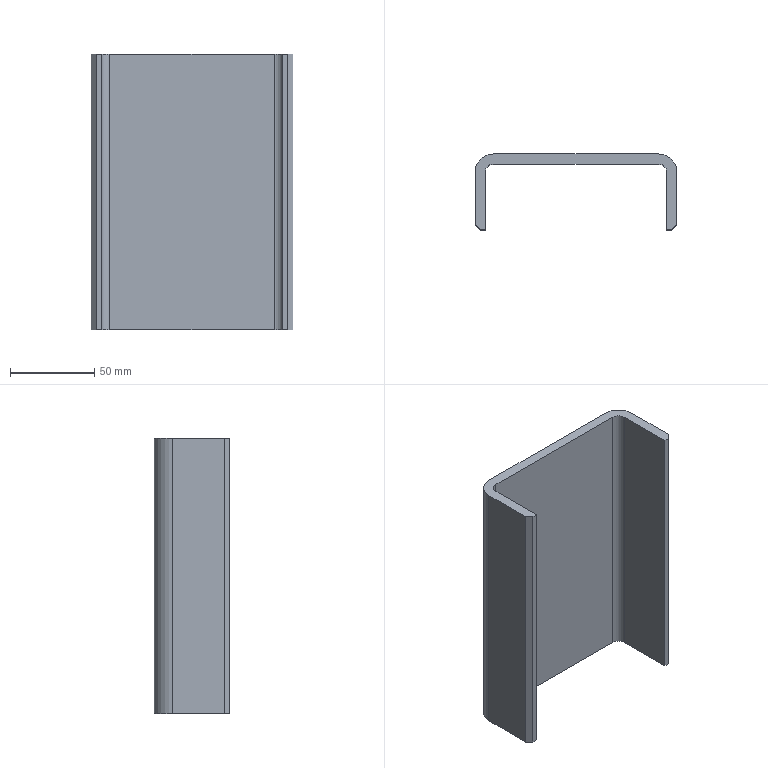Part | STEP file | VD-SYL0380DJ1006_1_1_2-2_VD-SYL | 1 solid | 16 faces | box 120 x 45 x 164 mm | volume 186599 mm3 | plane 12 | cylinder 4 | commonest cylinder face diameters 10 x2 22 x2
STEP:
#1=CARTESIAN_POINT('',(-49.,22.5,82.));
#2=VERTEX_POINT('',#1);
#3=CARTESIAN_POINT('',(-49.,22.5,-82.));
#4=VERTEX_POINT('',#3);
#5=CARTESIAN_POINT('',(-49.,22.5,82.));
#6=DIRECTION('',(0.,0.,-1.));
#7=VECTOR('',#6,1000.);
#8=LINE('',#5,#7);
#9=EDGE_CURVE('',#2,#4,#8,.T.);
#10=ORIENTED_EDGE('',*,*,#9,.T.);
#11=CARTESIAN_POINT('',(-60.,11.5,-82.));
#12=VERTEX_POINT('',#11);
#13=CARTESIAN_POINT('',(-49.,11.5,-82.));
#14=DIRECTION('',(0.,0.,-1.));
#15=DIRECTION('',(-1.,0.,0.));
#16=AXIS2_PLACEMENT_3D('',#13,#14,#15);
#17=CIRCLE('',#16,11.);
#18=EDGE_CURVE('',#12,#4,#17,.T.);
#19=ORIENTED_EDGE('',*,*,#18,.F.);
#20=CARTESIAN_POINT('',(-60.,11.5,82.));
#21=VERTEX_POINT('',#20);
#22=CARTESIAN_POINT('',(-60.,11.5,-82.));
#23=DIRECTION('',(0.,0.,1.));
#24=VECTOR('',#23,1000.);
#25=LINE('',#22,#24);
#26=EDGE_CURVE('',#12,#21,#25,.T.);
#27=ORIENTED_EDGE('',*,*,#26,.T.);
#28=CARTESIAN_POINT('',(-49.,11.5,82.));
#29=DIRECTION('',(0.,0.,1.));
#30=DIRECTION('',(0.,1.,0.));
#31=AXIS2_PLACEMENT_3D('',#28,#29,#30);
#32=CIRCLE('',#31,11.);
#33=EDGE_CURVE('',#2,#21,#32,.T.);
#34=ORIENTED_EDGE('',*,*,#33,.F.);
#35=EDGE_LOOP('',(#10,#19,#27,#34));
#36=FACE_OUTER_BOUND('',#35,.T.);
#37=CARTESIAN_POINT('',(-49.,11.5,295.79));
#38=DIRECTION('',(0.,0.,-1.));
#39=DIRECTION('',(-1.,0.,0.));
#40=AXIS2_PLACEMENT_3D('',#37,#38,#39);
#41=CYLINDRICAL_SURFACE('',#40,11.);
#42=ADVANCED_FACE('',(#36),#41,.T.);
#43=CARTESIAN_POINT('',(-60.,-19.5,82.));
#44=VERTEX_POINT('',#43);
#45=CARTESIAN_POINT('',(-60.,-19.5,-82.));
#46=VERTEX_POINT('',#45);
#47=CARTESIAN_POINT('',(-60.,-19.5,82.));
#48=DIRECTION('',(0.,0.,-1.));
#49=VECTOR('',#48,1000.);
#50=LINE('',#47,#49);
#51=EDGE_CURVE('',#44,#46,#50,.T.);
#52=ORIENTED_EDGE('',*,*,#51,.F.);
#53=CARTESIAN_POINT('',(-60.,11.5,82.));
#54=DIRECTION('',(0.,-1.,0.));
#55=VECTOR('',#54,1000.);
#56=LINE('',#53,#55);
#57=EDGE_CURVE('',#21,#44,#56,.T.);
#58=ORIENTED_EDGE('',*,*,#57,.F.);
#59=ORIENTED_EDGE('',*,*,#26,.F.);
#60=CARTESIAN_POINT('',(-60.,-19.5,-82.));
#61=DIRECTION('',(0.,1.,0.));
#62=VECTOR('',#61,1000.);
#63=LINE('',#60,#62);
#64=EDGE_CURVE('',#46,#12,#63,.T.);
#65=ORIENTED_EDGE('',*,*,#64,.F.);
#66=EDGE_LOOP('',(#52,#58,#59,#65));
#67=FACE_OUTER_BOUND('',#66,.T.);
#68=CARTESIAN_POINT('',(-60.,22.5,-82.));
#69=DIRECTION('',(-1.,0.,0.));
#70=DIRECTION('',(0.,0.,1.));
#71=AXIS2_PLACEMENT_3D('',#68,#69,#70);
#72=PLANE('',#71);
#73=ADVANCED_FACE('',(#67),#72,.T.);
#74=CARTESIAN_POINT('',(-57.,-22.5,-82.));
#75=VERTEX_POINT('',#74);
#76=CARTESIAN_POINT('',(-57.,-22.5,-82.));
#77=DIRECTION('',(-0.7071,0.7071,0.));
#78=VECTOR('',#77,1000.);
#79=LINE('',#76,#78);
#80=EDGE_CURVE('',#75,#46,#79,.T.);
#81=ORIENTED_EDGE('',*,*,#80,.F.);
#82=CARTESIAN_POINT('',(-57.,-22.5,82.));
#83=VERTEX_POINT('',#82);
#84=CARTESIAN_POINT('',(-57.,-22.5,82.));
#85=DIRECTION('',(0.,0.,-1.));
#86=VECTOR('',#85,1000.);
#87=LINE('',#84,#86);
#88=EDGE_CURVE('',#83,#75,#87,.T.);
#89=ORIENTED_EDGE('',*,*,#88,.F.);
#90=CARTESIAN_POINT('',(-60.,-19.5,82.));
#91=DIRECTION('',(0.7071,-0.7071,0.));
#92=VECTOR('',#91,1000.);
#93=LINE('',#90,#92);
#94=EDGE_CURVE('',#44,#83,#93,.T.);
#95=ORIENTED_EDGE('',*,*,#94,.F.);
#96=ORIENTED_EDGE('',*,*,#51,.T.);
#97=EDGE_LOOP('',(#81,#89,#95,#96));
#98=FACE_OUTER_BOUND('',#97,.T.);
#99=CARTESIAN_POINT('',(-58.5,-21.,0.));
#100=DIRECTION('',(-0.7071,-0.7071,0.));
#101=DIRECTION('',(-0.7071,0.7071,0.));
#102=AXIS2_PLACEMENT_3D('',#99,#100,#101);
#103=PLANE('',#102);
#104=ADVANCED_FACE('',(#98),#103,.T.);
#105=ORIENTED_EDGE('',*,*,#88,.T.);
#106=CARTESIAN_POINT('',(-54.,-22.5,-82.));
#107=VERTEX_POINT('',#106);
#108=CARTESIAN_POINT('',(-57.,-22.5,-82.));
#109=DIRECTION('',(1.,0.,0.));
#110=VECTOR('',#109,1000.);
#111=LINE('',#108,#110);
#112=EDGE_CURVE('',#75,#107,#111,.T.);
#113=ORIENTED_EDGE('',*,*,#112,.T.);
#114=CARTESIAN_POINT('',(-54.,-22.5,82.));
#115=VERTEX_POINT('',#114);
#116=CARTESIAN_POINT('',(-54.,-22.5,82.));
#117=DIRECTION('',(0.,0.,-1.));
#118=VECTOR('',#117,1000.);
#119=LINE('',#116,#118);
#120=EDGE_CURVE('',#115,#107,#119,.T.);
#121=ORIENTED_EDGE('',*,*,#120,.F.);
#122=CARTESIAN_POINT('',(-57.,-22.5,82.));
#123=DIRECTION('',(1.,0.,0.));
#124=VECTOR('',#123,1000.);
#125=LINE('',#122,#124);
#126=EDGE_CURVE('',#83,#115,#125,.T.);
#127=ORIENTED_EDGE('',*,*,#126,.F.);
#128=EDGE_LOOP('',(#105,#113,#121,#127));
#129=FACE_OUTER_BOUND('',#128,.T.);
#130=CARTESIAN_POINT('',(-57.,-22.5,0.));
#131=DIRECTION('',(0.,-1.,0.));
#132=DIRECTION('',(0.,0.,-1.));
#133=AXIS2_PLACEMENT_3D('',#130,#131,#132);
#134=PLANE('',#133);
#135=ADVANCED_FACE('',(#129),#134,.T.);
#136=CARTESIAN_POINT('',(-54.,11.5,-82.));
#137=VERTEX_POINT('',#136);
#138=CARTESIAN_POINT('',(-54.,-22.5,-82.));
#139=DIRECTION('',(0.,1.,0.));
#140=VECTOR('',#139,1000.);
#141=LINE('',#138,#140);
#142=EDGE_CURVE('',#107,#137,#141,.T.);
#143=ORIENTED_EDGE('',*,*,#142,.T.);
#144=CARTESIAN_POINT('',(-54.,11.5,82.));
#145=VERTEX_POINT('',#144);
#146=CARTESIAN_POINT('',(-54.,11.5,82.));
#147=DIRECTION('',(0.,0.,-1.));
#148=VECTOR('',#147,1000.);
#149=LINE('',#146,#148);
#150=EDGE_CURVE('',#145,#137,#149,.T.);
#151=ORIENTED_EDGE('',*,*,#150,.F.);
#152=CARTESIAN_POINT('',(-54.,-22.5,82.));
#153=DIRECTION('',(0.,1.,0.));
#154=VECTOR('',#153,1000.);
#155=LINE('',#152,#154);
#156=EDGE_CURVE('',#115,#145,#155,.T.);
#157=ORIENTED_EDGE('',*,*,#156,.F.);
#158=ORIENTED_EDGE('',*,*,#120,.T.);
#159=EDGE_LOOP('',(#143,#151,#157,#158));
#160=FACE_OUTER_BOUND('',#159,.T.);
#161=CARTESIAN_POINT('',(-54.,22.5,-82.));
#162=DIRECTION('',(-1.,0.,0.));
#163=DIRECTION('',(0.,0.,1.));
#164=AXIS2_PLACEMENT_3D('',#161,#162,#163);
#165=PLANE('',#164);
#166=ADVANCED_FACE('',(#160),#165,.F.);
#167=CARTESIAN_POINT('',(-49.,16.5,-82.));
#168=VERTEX_POINT('',#167);
#169=CARTESIAN_POINT('',(-49.,11.5,-82.));
#170=DIRECTION('',(0.,0.,1.));
#171=DIRECTION('',(0.,1.,0.));
#172=AXIS2_PLACEMENT_3D('',#169,#170,#171);
#173=CIRCLE('',#172,5.);
#174=EDGE_CURVE('',#168,#137,#173,.T.);
#175=ORIENTED_EDGE('',*,*,#174,.F.);
#176=CARTESIAN_POINT('',(-49.,16.5,82.));
#177=VERTEX_POINT('',#176);
#178=CARTESIAN_POINT('',(-49.,16.5,-82.));
#179=DIRECTION('',(0.,0.,1.));
#180=VECTOR('',#179,1000.);
#181=LINE('',#178,#180);
#182=EDGE_CURVE('',#168,#177,#181,.T.);
#183=ORIENTED_EDGE('',*,*,#182,.T.);
#184=CARTESIAN_POINT('',(-49.,11.5,82.));
#185=DIRECTION('',(0.,0.,-1.));
#186=DIRECTION('',(-1.,0.,0.));
#187=AXIS2_PLACEMENT_3D('',#184,#185,#186);
#188=CIRCLE('',#187,5.);
#189=EDGE_CURVE('',#145,#177,#188,.T.);
#190=ORIENTED_EDGE('',*,*,#189,.F.);
#191=ORIENTED_EDGE('',*,*,#150,.T.);
#192=EDGE_LOOP('',(#175,#183,#190,#191));
#193=FACE_OUTER_BOUND('',#192,.T.);
#194=CARTESIAN_POINT('',(-49.,11.5,295.79));
#195=DIRECTION('',(0.,0.,-1.));
#196=DIRECTION('',(-1.,0.,0.));
#197=AXIS2_PLACEMENT_3D('',#194,#195,#196);
#198=CYLINDRICAL_SURFACE('',#197,5.);
#199=ADVANCED_FACE('',(#193),#198,.F.);
#200=CARTESIAN_POINT('',(54.,11.5,82.));
#201=VERTEX_POINT('',#200);
#202=CARTESIAN_POINT('',(54.,-22.5,82.));
#203=VERTEX_POINT('',#202);
#204=CARTESIAN_POINT('',(54.,11.5,82.));
#205=DIRECTION('',(0.,-1.,0.));
#206=VECTOR('',#205,1000.);
#207=LINE('',#204,#206);
#208=EDGE_CURVE('',#201,#203,#207,.T.);
#209=ORIENTED_EDGE('',*,*,#208,.F.);
#210=CARTESIAN_POINT('',(54.,11.5,-82.));
#211=VERTEX_POINT('',#210);
#212=CARTESIAN_POINT('',(54.,11.5,-82.));
#213=DIRECTION('',(0.,0.,1.));
#214=VECTOR('',#213,1000.);
#215=LINE('',#212,#214);
#216=EDGE_CURVE('',#211,#201,#215,.T.);
#217=ORIENTED_EDGE('',*,*,#216,.F.);
#218=CARTESIAN_POINT('',(54.,-22.5,-82.));
#219=VERTEX_POINT('',#218);
#220=CARTESIAN_POINT('',(54.,11.5,-82.));
#221=DIRECTION('',(0.,-1.,0.));
#222=VECTOR('',#221,1000.);
#223=LINE('',#220,#222);
#224=EDGE_CURVE('',#211,#219,#223,.T.);
#225=ORIENTED_EDGE('',*,*,#224,.T.);
#226=CARTESIAN_POINT('',(54.,-22.5,-82.));
#227=DIRECTION('',(0.,0.,1.));
#228=VECTOR('',#227,1000.);
#229=LINE('',#226,#228);
#230=EDGE_CURVE('',#219,#203,#229,.T.);
#231=ORIENTED_EDGE('',*,*,#230,.T.);
#232=EDGE_LOOP('',(#209,#217,#225,#231));
#233=FACE_OUTER_BOUND('',#232,.T.);
#234=CARTESIAN_POINT('',(54.,-22.5,-82.));
#235=DIRECTION('',(1.,0.,0.));
#236=DIRECTION('',(0.,1.,0.));
#237=AXIS2_PLACEMENT_3D('',#234,#235,#236);
#238=PLANE('',#237);
#239=ADVANCED_FACE('',(#233),#238,.F.);
#240=CARTESIAN_POINT('',(57.,-22.5,-82.));
#241=VERTEX_POINT('',#240);
#242=CARTESIAN_POINT('',(54.,-22.5,-82.));
#243=DIRECTION('',(1.,0.,0.));
#244=VECTOR('',#243,1000.);
#245=LINE('',#242,#244);
#246=EDGE_CURVE('',#219,#241,#245,.T.);
#247=ORIENTED_EDGE('',*,*,#246,.T.);
#248=CARTESIAN_POINT('',(57.,-22.5,82.));
#249=VERTEX_POINT('',#248);
#250=CARTESIAN_POINT('',(57.,-22.5,-82.));
#251=DIRECTION('',(0.,0.,1.));
#252=VECTOR('',#251,1000.);
#253=LINE('',#250,#252);
#254=EDGE_CURVE('',#241,#249,#253,.T.);
#255=ORIENTED_EDGE('',*,*,#254,.T.);
#256=CARTESIAN_POINT('',(54.,-22.5,82.));
#257=DIRECTION('',(1.,0.,0.));
#258=VECTOR('',#257,1000.);
#259=LINE('',#256,#258);
#260=EDGE_CURVE('',#203,#249,#259,.T.);
#261=ORIENTED_EDGE('',*,*,#260,.F.);
#262=ORIENTED_EDGE('',*,*,#230,.F.);
#263=EDGE_LOOP('',(#247,#255,#261,#262));
#264=FACE_OUTER_BOUND('',#263,.T.);
#265=CARTESIAN_POINT('',(57.,-22.5,0.));
#266=DIRECTION('',(0.,1.,0.));
#267=DIRECTION('',(1.,0.,0.));
#268=AXIS2_PLACEMENT_3D('',#265,#266,#267);
#269=PLANE('',#268);
#270=ADVANCED_FACE('',(#264),#269,.F.);
#271=CARTESIAN_POINT('',(60.,-19.5,-82.));
#272=VERTEX_POINT('',#271);
#273=CARTESIAN_POINT('',(60.,-19.5,-82.));
#274=DIRECTION('',(-0.7071,-0.7071,0.));
#275=VECTOR('',#274,1000.);
#276=LINE('',#273,#275);
#277=EDGE_CURVE('',#272,#241,#276,.T.);
#278=ORIENTED_EDGE('',*,*,#277,.F.);
#279=CARTESIAN_POINT('',(60.,-19.5,82.));
#280=VERTEX_POINT('',#279);
#281=CARTESIAN_POINT('',(60.,-19.5,-82.));
#282=DIRECTION('',(0.,0.,1.));
#283=VECTOR('',#282,1000.);
#284=LINE('',#281,#283);
#285=EDGE_CURVE('',#272,#280,#284,.T.);
#286=ORIENTED_EDGE('',*,*,#285,.T.);
#287=CARTESIAN_POINT('',(57.,-22.5,82.));
#288=DIRECTION('',(0.7071,0.7071,0.));
#289=VECTOR('',#288,1000.);
#290=LINE('',#287,#289);
#291=EDGE_CURVE('',#249,#280,#290,.T.);
#292=ORIENTED_EDGE('',*,*,#291,.F.);
#293=ORIENTED_EDGE('',*,*,#254,.F.);
#294=EDGE_LOOP('',(#278,#286,#292,#293));
#295=FACE_OUTER_BOUND('',#294,.T.);
#296=CARTESIAN_POINT('',(58.5,-21.,0.));
#297=DIRECTION('',(0.7071,-0.7071,0.));
#298=DIRECTION('',(0.,0.,-1.));
#299=AXIS2_PLACEMENT_3D('',#296,#297,#298);
#300=PLANE('',#299);
#301=ADVANCED_FACE('',(#295),#300,.T.);
#302=ORIENTED_EDGE('',*,*,#285,.F.);
#303=CARTESIAN_POINT('',(60.,11.5,-82.));
#304=VERTEX_POINT('',#303);
#305=CARTESIAN_POINT('',(60.,11.5,-82.));
#306=DIRECTION('',(0.,-1.,0.));
#307=VECTOR('',#306,1000.);
#308=LINE('',#305,#307);
#309=EDGE_CURVE('',#304,#272,#308,.T.);
#310=ORIENTED_EDGE('',*,*,#309,.F.);
#311=CARTESIAN_POINT('',(60.,11.5,82.));
#312=VERTEX_POINT('',#311);
#313=CARTESIAN_POINT('',(60.,11.5,82.));
#314=DIRECTION('',(0.,0.,-1.));
#315=VECTOR('',#314,1000.);
#316=LINE('',#313,#315);
#317=EDGE_CURVE('',#312,#304,#316,.T.);
#318=ORIENTED_EDGE('',*,*,#317,.F.);
#319=CARTESIAN_POINT('',(60.,-19.5,82.));
#320=DIRECTION('',(0.,1.,0.));
#321=VECTOR('',#320,1000.);
#322=LINE('',#319,#321);
#323=EDGE_CURVE('',#280,#312,#322,.T.);
#324=ORIENTED_EDGE('',*,*,#323,.F.);
#325=EDGE_LOOP('',(#302,#310,#318,#324));
#326=FACE_OUTER_BOUND('',#325,.T.);
#327=CARTESIAN_POINT('',(60.,-22.5,-82.));
#328=DIRECTION('',(1.,0.,0.));
#329=DIRECTION('',(0.,1.,0.));
#330=AXIS2_PLACEMENT_3D('',#327,#328,#329);
#331=PLANE('',#330);
#332=ADVANCED_FACE('',(#326),#331,.T.);
#333=ORIENTED_EDGE('',*,*,#317,.T.);
#334=CARTESIAN_POINT('',(49.,22.5,-82.));
#335=VERTEX_POINT('',#334);
#336=CARTESIAN_POINT('',(49.,11.5,-82.));
#337=DIRECTION('',(0.,0.,-1.));
#338=DIRECTION('',(0.,1.,0.));
#339=AXIS2_PLACEMENT_3D('',#336,#337,#338);
#340=CIRCLE('',#339,11.);
#341=EDGE_CURVE('',#335,#304,#340,.T.);
#342=ORIENTED_EDGE('',*,*,#341,.F.);
#343=CARTESIAN_POINT('',(49.,22.5,82.));
#344=VERTEX_POINT('',#343);
#345=CARTESIAN_POINT('',(49.,22.5,-82.));
#346=DIRECTION('',(0.,0.,1.));
#347=VECTOR('',#346,1000.);
#348=LINE('',#345,#347);
#349=EDGE_CURVE('',#335,#344,#348,.T.);
#350=ORIENTED_EDGE('',*,*,#349,.T.);
#351=CARTESIAN_POINT('',(49.,11.5,82.));
#352=DIRECTION('',(0.,0.,1.));
#353=DIRECTION('',(1.,0.,0.));
#354=AXIS2_PLACEMENT_3D('',#351,#352,#353);
#355=CIRCLE('',#354,11.);
#356=EDGE_CURVE('',#312,#344,#355,.T.);
#357=ORIENTED_EDGE('',*,*,#356,.F.);
#358=EDGE_LOOP('',(#333,#342,#350,#357));
#359=FACE_OUTER_BOUND('',#358,.T.);
#360=CARTESIAN_POINT('',(49.,11.5,295.79));
#361=DIRECTION('',(0.,0.,-1.));
#362=DIRECTION('',(-1.,0.,0.));
#363=AXIS2_PLACEMENT_3D('',#360,#361,#362);
#364=CYLINDRICAL_SURFACE('',#363,11.);
#365=ADVANCED_FACE('',(#359),#364,.T.);
#366=ORIENTED_EDGE('',*,*,#33,.T.);
#367=ORIENTED_EDGE('',*,*,#57,.T.);
#368=ORIENTED_EDGE('',*,*,#94,.T.);
#369=ORIENTED_EDGE('',*,*,#126,.T.);
#370=ORIENTED_EDGE('',*,*,#156,.T.);
#371=ORIENTED_EDGE('',*,*,#189,.T.);
#372=CARTESIAN_POINT('',(49.,16.5,82.));
#373=VERTEX_POINT('',#372);
#374=CARTESIAN_POINT('',(-49.,16.5,82.));
#375=DIRECTION('',(1.,0.,0.));
#376=VECTOR('',#375,1000.);
#377=LINE('',#374,#376);
#378=EDGE_CURVE('',#177,#373,#377,.T.);
#379=ORIENTED_EDGE('',*,*,#378,.T.);
#380=CARTESIAN_POINT('',(49.,11.5,82.));
#381=DIRECTION('',(0.,0.,-1.));
#382=DIRECTION('',(0.,1.,0.));
#383=AXIS2_PLACEMENT_3D('',#380,#381,#382);
#384=CIRCLE('',#383,5.);
#385=EDGE_CURVE('',#373,#201,#384,.T.);
#386=ORIENTED_EDGE('',*,*,#385,.T.);
#387=ORIENTED_EDGE('',*,*,#208,.T.);
#388=ORIENTED_EDGE('',*,*,#260,.T.);
#389=ORIENTED_EDGE('',*,*,#291,.T.);
#390=ORIENTED_EDGE('',*,*,#323,.T.);
#391=ORIENTED_EDGE('',*,*,#356,.T.);
#392=CARTESIAN_POINT('',(49.,22.5,82.));
#393=DIRECTION('',(-1.,0.,0.));
#394=VECTOR('',#393,1000.);
#395=LINE('',#392,#394);
#396=EDGE_CURVE('',#344,#2,#395,.T.);
#397=ORIENTED_EDGE('',*,*,#396,.T.);
#398=EDGE_LOOP('',(#366,#367,#368,#369,#370,#371,#379,#386,#387,#388,#389,#390,#391,#397));
#399=FACE_OUTER_BOUND('',#398,.T.);
#400=CARTESIAN_POINT('',(0.,19.5,82.));
#401=DIRECTION('',(0.,0.,-1.));
#402=DIRECTION('',(0.,-1.,0.));
#403=AXIS2_PLACEMENT_3D('',#400,#401,#402);
#404=PLANE('',#403);
#405=ADVANCED_FACE('',(#399),#404,.F.);
#406=CARTESIAN_POINT('',(49.,16.5,-82.));
#407=VERTEX_POINT('',#406);
#408=CARTESIAN_POINT('',(49.,11.5,-82.));
#409=DIRECTION('',(0.,0.,1.));
#410=DIRECTION('',(1.,0.,0.));
#411=AXIS2_PLACEMENT_3D('',#408,#409,#410);
#412=CIRCLE('',#411,5.);
#413=EDGE_CURVE('',#211,#407,#412,.T.);
#414=ORIENTED_EDGE('',*,*,#413,.F.);
#415=ORIENTED_EDGE('',*,*,#216,.T.);
#416=ORIENTED_EDGE('',*,*,#385,.F.);
#417=CARTESIAN_POINT('',(49.,16.5,82.));
#418=DIRECTION('',(0.,0.,-1.));
#419=VECTOR('',#418,1000.);
#420=LINE('',#417,#419);
#421=EDGE_CURVE('',#373,#407,#420,.T.);
#422=ORIENTED_EDGE('',*,*,#421,.T.);
#423=EDGE_LOOP('',(#414,#415,#416,#422));
#424=FACE_OUTER_BOUND('',#423,.T.);
#425=CARTESIAN_POINT('',(49.,11.5,295.79));
#426=DIRECTION('',(0.,0.,-1.));
#427=DIRECTION('',(-1.,0.,0.));
#428=AXIS2_PLACEMENT_3D('',#425,#426,#427);
#429=CYLINDRICAL_SURFACE('',#428,5.);
#430=ADVANCED_FACE('',(#424),#429,.F.);
#431=ORIENTED_EDGE('',*,*,#378,.F.);
#432=ORIENTED_EDGE('',*,*,#182,.F.);
#433=CARTESIAN_POINT('',(-49.,16.5,-82.));
#434=DIRECTION('',(1.,0.,0.));
#435=VECTOR('',#434,1000.);
#436=LINE('',#433,#435);
#437=EDGE_CURVE('',#168,#407,#436,.T.);
#438=ORIENTED_EDGE('',*,*,#437,.T.);
#439=ORIENTED_EDGE('',*,*,#421,.F.);
#440=EDGE_LOOP('',(#431,#432,#438,#439));
#441=FACE_OUTER_BOUND('',#440,.T.);
#442=CARTESIAN_POINT('',(60.,16.5,-82.));
#443=DIRECTION('',(0.,1.,0.));
#444=DIRECTION('',(1.,0.,0.));
#445=AXIS2_PLACEMENT_3D('',#442,#443,#444);
#446=PLANE('',#445);
#447=ADVANCED_FACE('',(#441),#446,.F.);
#448=ORIENTED_EDGE('',*,*,#174,.T.);
#449=ORIENTED_EDGE('',*,*,#142,.F.);
#450=ORIENTED_EDGE('',*,*,#112,.F.);
#451=ORIENTED_EDGE('',*,*,#80,.T.);
#452=ORIENTED_EDGE('',*,*,#64,.T.);
#453=ORIENTED_EDGE('',*,*,#18,.T.);
#454=CARTESIAN_POINT('',(-49.,22.5,-82.));
#455=DIRECTION('',(1.,0.,0.));
#456=VECTOR('',#455,1000.);
#457=LINE('',#454,#456);
#458=EDGE_CURVE('',#4,#335,#457,.T.);
#459=ORIENTED_EDGE('',*,*,#458,.T.);
#460=ORIENTED_EDGE('',*,*,#341,.T.);
#461=ORIENTED_EDGE('',*,*,#309,.T.);
#462=ORIENTED_EDGE('',*,*,#277,.T.);
#463=ORIENTED_EDGE('',*,*,#246,.F.);
#464=ORIENTED_EDGE('',*,*,#224,.F.);
#465=ORIENTED_EDGE('',*,*,#413,.T.);
#466=ORIENTED_EDGE('',*,*,#437,.F.);
#467=EDGE_LOOP('',(#448,#449,#450,#451,#452,#453,#459,#460,#461,#462,#463,#464,#465,#466));
#468=FACE_OUTER_BOUND('',#467,.T.);
#469=CARTESIAN_POINT('',(0.,19.5,-82.));
#470=DIRECTION('',(0.,0.,-1.));
#471=DIRECTION('',(0.,-1.,0.));
#472=AXIS2_PLACEMENT_3D('',#469,#470,#471);
#473=PLANE('',#472);
#474=ADVANCED_FACE('',(#468),#473,.T.);
#475=ORIENTED_EDGE('',*,*,#9,.F.);
#476=ORIENTED_EDGE('',*,*,#396,.F.);
#477=ORIENTED_EDGE('',*,*,#349,.F.);
#478=ORIENTED_EDGE('',*,*,#458,.F.);
#479=EDGE_LOOP('',(#475,#476,#477,#478));
#480=FACE_OUTER_BOUND('',#479,.T.);
#481=CARTESIAN_POINT('',(60.,22.5,-82.));
#482=DIRECTION('',(0.,1.,0.));
#483=DIRECTION('',(1.,0.,0.));
#484=AXIS2_PLACEMENT_3D('',#481,#482,#483);
#485=PLANE('',#484);
#486=ADVANCED_FACE('',(#480),#485,.T.);
#487=CLOSED_SHELL('',(#42,#73,#104,#135,#166,#199,#239,#270,#301,#332,#365,#405,#430,#447,#474,#486));
#488=MANIFOLD_SOLID_BREP('',#487);
#489=CARTESIAN_POINT('',(0.,0.,0.));
#490=DIRECTION('',(0.,0.,1.));
#491=DIRECTION('',(1.,0.,0.));
#492=AXIS2_PLACEMENT_3D('',#489,#490,#491);
#493=(LENGTH_UNIT()NAMED_UNIT(*)SI_UNIT(.MILLI.,.METRE.));
#494=UNCERTAINTY_MEASURE_WITH_UNIT(LENGTH_MEASURE(0.00001),#493,'','');
#495=(NAMED_UNIT(*)PLANE_ANGLE_UNIT()SI_UNIT($,.RADIAN.));
#496=(NAMED_UNIT(*)SI_UNIT($,.STERADIAN.)SOLID_ANGLE_UNIT());
#497=(GEOMETRIC_REPRESENTATION_CONTEXT(3)GLOBAL_UNCERTAINTY_ASSIGNED_CONTEXT((#494))GLOBAL_UNIT_ASSIGNED_CONTEXT((#493,#495,#496))REPRESENTATION_CONTEXT('',''));
#498=ADVANCED_BREP_SHAPE_REPRESENTATION('',(#488,#492),#497);